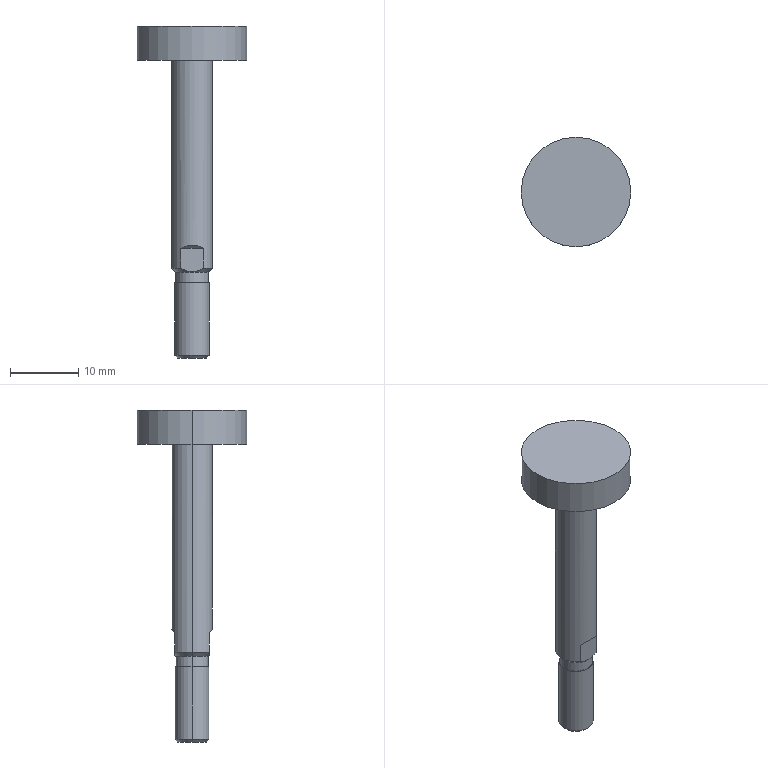Part | NX | features BREP 1 | 1 solid | 20 faces | box 16 x 16 x 48.5 mm | volume 2113 mm3 | cylinder 8 | plane 8 | cone 4 | commonest cylinder face diameters 4.8 x2 5 x2 6 x2 16 x2
STEP:
#1=CARTESIAN_POINT('',(2.1,0.,-43.5));
#2=VERTEX_POINT('',#1);
#3=CARTESIAN_POINT('',(-2.1,0.,-43.5));
#4=VERTEX_POINT('',#3);
#5=CARTESIAN_POINT('',(0.,0.,-43.5));
#6=DIRECTION('',(0.,0.,1.));
#7=DIRECTION('',(1.,0.,0.));
#8=AXIS2_PLACEMENT_3D('',#5,#6,#7);
#9=CIRCLE('',#8,2.1);
#10=EDGE_CURVE('',#2,#4,#9,.T.);
#11=ORIENTED_EDGE('',*,*,#10,.T.);
#12=CARTESIAN_POINT('',(-2.5,0.,-43.1));
#13=VERTEX_POINT('',#12);
#14=CARTESIAN_POINT('',(-2.5,0.,-43.1));
#15=DIRECTION('',(-0.7071,0.,0.7071));
#16=VECTOR('',#15,1000.);
#17=LINE('',#14,#16);
#18=EDGE_CURVE('',#13,#4,#17,.F.);
#19=ORIENTED_EDGE('',*,*,#18,.F.);
#20=CARTESIAN_POINT('',(2.5,0.,-43.1));
#21=VERTEX_POINT('',#20);
#22=CARTESIAN_POINT('',(0.,0.,-43.1));
#23=DIRECTION('',(0.,0.,1.));
#24=DIRECTION('',(1.,0.,0.));
#25=AXIS2_PLACEMENT_3D('',#22,#23,#24);
#26=CIRCLE('',#25,2.5);
#27=EDGE_CURVE('',#21,#13,#26,.T.);
#28=ORIENTED_EDGE('',*,*,#27,.F.);
#29=CARTESIAN_POINT('',(2.5,0.,-43.1));
#30=DIRECTION('',(0.7071,0.,0.7071));
#31=VECTOR('',#30,1000.);
#32=LINE('',#29,#31);
#33=EDGE_CURVE('',#21,#2,#32,.F.);
#34=ORIENTED_EDGE('',*,*,#33,.T.);
#35=EDGE_LOOP('',(#11,#19,#28,#34));
#36=FACE_BOUND('',#35,.T.);
#37=CARTESIAN_POINT('',(0.,0.,-43.1));
#38=DIRECTION('',(0.,0.,1.));
#39=DIRECTION('',(1.,0.,0.));
#40=AXIS2_PLACEMENT_3D('',#37,#38,#39);
#41=CONICAL_SURFACE('',#40,2.5,0.7854);
#42=ADVANCED_FACE('',(#36),#41,.T.);
#43=ORIENTED_EDGE('',*,*,#27,.T.);
#44=CARTESIAN_POINT('',(-2.5,0.,-32.5));
#45=VERTEX_POINT('',#44);
#46=CARTESIAN_POINT('',(-2.5,0.,0.));
#47=DIRECTION('',(0.,0.,1.));
#48=VECTOR('',#47,1000.);
#49=LINE('',#46,#48);
#50=EDGE_CURVE('',#45,#13,#49,.F.);
#51=ORIENTED_EDGE('',*,*,#50,.F.);
#52=CARTESIAN_POINT('',(2.5,0.,-32.5));
#53=VERTEX_POINT('',#52);
#54=CARTESIAN_POINT('',(0.,0.,-32.5));
#55=DIRECTION('',(0.,0.,1.));
#56=DIRECTION('',(1.,0.,0.));
#57=AXIS2_PLACEMENT_3D('',#54,#55,#56);
#58=CIRCLE('',#57,2.5);
#59=EDGE_CURVE('',#53,#45,#58,.T.);
#60=ORIENTED_EDGE('',*,*,#59,.F.);
#61=CARTESIAN_POINT('',(2.5,0.,0.));
#62=DIRECTION('',(0.,0.,1.));
#63=VECTOR('',#62,1000.);
#64=LINE('',#61,#63);
#65=EDGE_CURVE('',#53,#21,#64,.F.);
#66=ORIENTED_EDGE('',*,*,#65,.T.);
#67=EDGE_LOOP('',(#43,#51,#60,#66));
#68=FACE_BOUND('',#67,.T.);
#69=CARTESIAN_POINT('',(0.,0.,0.));
#70=DIRECTION('',(0.,0.,1.));
#71=DIRECTION('',(1.,0.,0.));
#72=AXIS2_PLACEMENT_3D('',#69,#70,#71);
#73=CYLINDRICAL_SURFACE('',#72,2.5);
#74=ADVANCED_FACE('',(#68),#73,.T.);
#75=CARTESIAN_POINT('',(2.4,0.,-32.5));
#76=VERTEX_POINT('',#75);
#77=CARTESIAN_POINT('',(-2.4,0.,-32.5));
#78=VERTEX_POINT('',#77);
#79=CARTESIAN_POINT('',(0.,0.,-32.5));
#80=DIRECTION('',(0.,0.,1.));
#81=DIRECTION('',(1.,0.,0.));
#82=AXIS2_PLACEMENT_3D('',#79,#80,#81);
#83=CIRCLE('',#82,2.4);
#84=EDGE_CURVE('',#76,#78,#83,.T.);
#85=ORIENTED_EDGE('',*,*,#84,.T.);
#86=CARTESIAN_POINT('',(-2.4,0.,-31.));
#87=VERTEX_POINT('',#86);
#88=CARTESIAN_POINT('',(-2.4,0.,0.));
#89=DIRECTION('',(0.,0.,1.));
#90=VECTOR('',#89,1000.);
#91=LINE('',#88,#90);
#92=EDGE_CURVE('',#87,#78,#91,.F.);
#93=ORIENTED_EDGE('',*,*,#92,.F.);
#94=CARTESIAN_POINT('',(2.4,0.,-31.));
#95=VERTEX_POINT('',#94);
#96=CARTESIAN_POINT('',(0.,0.,-31.));
#97=DIRECTION('',(0.,0.,1.));
#98=DIRECTION('',(1.,0.,0.));
#99=AXIS2_PLACEMENT_3D('',#96,#97,#98);
#100=CIRCLE('',#99,2.4);
#101=EDGE_CURVE('',#95,#87,#100,.T.);
#102=ORIENTED_EDGE('',*,*,#101,.F.);
#103=CARTESIAN_POINT('',(2.4,0.,0.));
#104=DIRECTION('',(0.,0.,1.));
#105=VECTOR('',#104,1000.);
#106=LINE('',#103,#105);
#107=EDGE_CURVE('',#95,#76,#106,.F.);
#108=ORIENTED_EDGE('',*,*,#107,.T.);
#109=EDGE_LOOP('',(#85,#93,#102,#108));
#110=FACE_BOUND('',#109,.T.);
#111=CARTESIAN_POINT('',(0.,0.,0.));
#112=DIRECTION('',(0.,0.,1.));
#113=DIRECTION('',(1.,0.,0.));
#114=AXIS2_PLACEMENT_3D('',#111,#112,#113);
#115=CYLINDRICAL_SURFACE('',#114,2.4);
#116=ADVANCED_FACE('',(#110),#115,.T.);
#117=ORIENTED_EDGE('',*,*,#101,.T.);
#118=CARTESIAN_POINT('',(-3.,0.,-30.4));
#119=VERTEX_POINT('',#118);
#120=CARTESIAN_POINT('',(-8.,0.,-25.4));
#121=DIRECTION('',(-0.7071,0.,0.7071));
#122=VECTOR('',#121,1000.);
#123=LINE('',#120,#122);
#124=EDGE_CURVE('',#119,#87,#123,.F.);
#125=ORIENTED_EDGE('',*,*,#124,.F.);
#126=CARTESIAN_POINT('',(-1.658,2.5,-30.4));
#127=VERTEX_POINT('',#126);
#128=CARTESIAN_POINT('',(0.,0.,-30.4));
#129=DIRECTION('',(0.,0.,1.));
#130=DIRECTION('',(1.,0.,0.));
#131=AXIS2_PLACEMENT_3D('',#128,#129,#130);
#132=CIRCLE('',#131,3.);
#133=EDGE_CURVE('',#127,#119,#132,.T.);
#134=ORIENTED_EDGE('',*,*,#133,.F.);
#135=CARTESIAN_POINT('',(1.658,2.5,-30.4));
#136=VERTEX_POINT('',#135);
#137=CARTESIAN_POINT('',(1.658,2.5,-30.4));
#138=CARTESIAN_POINT('',(1.376,2.5,-30.556));
#139=CARTESIAN_POINT('',(0.8861,2.5,-30.784));
#140=CARTESIAN_POINT('',(-0.001734,2.5,-30.958));
#141=CARTESIAN_POINT('',(-0.8871,2.5,-30.783));
#142=CARTESIAN_POINT('',(-1.376,2.5,-30.556));
#143=CARTESIAN_POINT('',(-1.658,2.5,-30.4));
#144=B_SPLINE_CURVE_WITH_KNOTS('',3,(#137,#138,#139,#140,#141,#142,#143),.UNSPECIFIED.,.F.,.F.,(4,1,1,1,4),(0.,0.25,0.5,0.75,1.),.UNSPECIFIED.);
#145=EDGE_CURVE('',#136,#127,#144,.T.);
#146=ORIENTED_EDGE('',*,*,#145,.F.);
#147=CARTESIAN_POINT('',(3.,0.,-30.4));
#148=VERTEX_POINT('',#147);
#149=CARTESIAN_POINT('',(0.,0.,-30.4));
#150=DIRECTION('',(0.,0.,1.));
#151=DIRECTION('',(1.,0.,0.));
#152=AXIS2_PLACEMENT_3D('',#149,#150,#151);
#153=CIRCLE('',#152,3.);
#154=EDGE_CURVE('',#148,#136,#153,.T.);
#155=ORIENTED_EDGE('',*,*,#154,.F.);
#156=CARTESIAN_POINT('',(8.,0.,-25.4));
#157=DIRECTION('',(0.7071,0.,0.7071));
#158=VECTOR('',#157,1000.);
#159=LINE('',#156,#158);
#160=EDGE_CURVE('',#148,#95,#159,.F.);
#161=ORIENTED_EDGE('',*,*,#160,.T.);
#162=EDGE_LOOP('',(#117,#125,#134,#146,#155,#161));
#163=FACE_BOUND('',#162,.T.);
#164=CARTESIAN_POINT('',(0.,0.,-25.4));
#165=DIRECTION('',(0.,0.,1.));
#166=DIRECTION('',(1.,0.,0.));
#167=AXIS2_PLACEMENT_3D('',#164,#165,#166);
#168=CONICAL_SURFACE('',#167,8.,0.7854);
#169=ADVANCED_FACE('',(#163),#168,.T.);
#170=CARTESIAN_POINT('',(8.,0.,5.));
#171=VERTEX_POINT('',#170);
#172=CARTESIAN_POINT('',(-8.,0.,5.));
#173=VERTEX_POINT('',#172);
#174=CARTESIAN_POINT('',(0.,0.,5.));
#175=DIRECTION('',(0.,0.,1.));
#176=DIRECTION('',(1.,0.,0.));
#177=AXIS2_PLACEMENT_3D('',#174,#175,#176);
#178=CIRCLE('',#177,8.);
#179=EDGE_CURVE('',#171,#173,#178,.T.);
#180=ORIENTED_EDGE('',*,*,#179,.F.);
#181=CARTESIAN_POINT('',(8.,0.,0.));
#182=VERTEX_POINT('',#181);
#183=CARTESIAN_POINT('',(8.,0.,5.));
#184=DIRECTION('',(0.,0.,-1.));
#185=VECTOR('',#184,1000.);
#186=LINE('',#183,#185);
#187=EDGE_CURVE('',#171,#182,#186,.T.);
#188=ORIENTED_EDGE('',*,*,#187,.T.);
#189=CARTESIAN_POINT('',(-8.,0.,0.));
#190=VERTEX_POINT('',#189);
#191=CARTESIAN_POINT('',(0.,0.,0.));
#192=DIRECTION('',(0.,0.,1.));
#193=DIRECTION('',(1.,0.,0.));
#194=AXIS2_PLACEMENT_3D('',#191,#192,#193);
#195=CIRCLE('',#194,8.);
#196=EDGE_CURVE('',#182,#190,#195,.T.);
#197=ORIENTED_EDGE('',*,*,#196,.T.);
#198=CARTESIAN_POINT('',(-8.,0.,5.));
#199=DIRECTION('',(0.,0.,-1.));
#200=VECTOR('',#199,1000.);
#201=LINE('',#198,#200);
#202=EDGE_CURVE('',#173,#190,#201,.T.);
#203=ORIENTED_EDGE('',*,*,#202,.F.);
#204=EDGE_LOOP('',(#180,#188,#197,#203));
#205=FACE_BOUND('',#204,.T.);
#206=CARTESIAN_POINT('',(0.,0.,5.));
#207=DIRECTION('',(0.,0.,-1.));
#208=DIRECTION('',(-1.,0.,0.));
#209=AXIS2_PLACEMENT_3D('',#206,#207,#208);
#210=CYLINDRICAL_SURFACE('',#209,8.);
#211=ADVANCED_FACE('',(#205),#210,.T.);
#212=ORIENTED_EDGE('',*,*,#133,.T.);
#213=CARTESIAN_POINT('',(-3.,0.,0.));
#214=VERTEX_POINT('',#213);
#215=CARTESIAN_POINT('',(-3.,0.,-51.985));
#216=DIRECTION('',(0.,0.,1.));
#217=VECTOR('',#216,1000.);
#218=LINE('',#215,#217);
#219=EDGE_CURVE('',#214,#119,#218,.F.);
#220=ORIENTED_EDGE('',*,*,#219,.F.);
#221=CARTESIAN_POINT('',(3.,0.,0.));
#222=VERTEX_POINT('',#221);
#223=CARTESIAN_POINT('',(0.,0.,0.));
#224=DIRECTION('',(0.,0.,1.));
#225=DIRECTION('',(1.,0.,0.));
#226=AXIS2_PLACEMENT_3D('',#223,#224,#225);
#227=CIRCLE('',#226,3.);
#228=EDGE_CURVE('',#222,#214,#227,.T.);
#229=ORIENTED_EDGE('',*,*,#228,.F.);
#230=CARTESIAN_POINT('',(3.,0.,-51.985));
#231=DIRECTION('',(0.,0.,1.));
#232=VECTOR('',#231,1000.);
#233=LINE('',#230,#232);
#234=EDGE_CURVE('',#222,#148,#233,.F.);
#235=ORIENTED_EDGE('',*,*,#234,.T.);
#236=ORIENTED_EDGE('',*,*,#154,.T.);
#237=CARTESIAN_POINT('',(1.658,2.5,-27.5));
#238=VERTEX_POINT('',#237);
#239=CARTESIAN_POINT('',(1.658,2.5,-51.985));
#240=DIRECTION('',(0.,0.,-1.));
#241=VECTOR('',#240,1000.);
#242=LINE('',#239,#241);
#243=EDGE_CURVE('',#238,#136,#242,.T.);
#244=ORIENTED_EDGE('',*,*,#243,.F.);
#245=CARTESIAN_POINT('',(-1.658,2.5,-27.5));
#246=VERTEX_POINT('',#245);
#247=CARTESIAN_POINT('',(-1.658,2.5,-27.5));
#248=CARTESIAN_POINT('',(-0.6219,3.188,-26.812));
#249=CARTESIAN_POINT('',(0.6219,3.188,-26.812));
#250=CARTESIAN_POINT('',(1.658,2.5,-27.5));
#251=(BOUNDED_CURVE()B_SPLINE_CURVE(3,(#247,#248,#249,#250),.UNSPECIFIED.,.F.,.F.)B_SPLINE_CURVE_WITH_KNOTS((4,4),(5.697,6.869),.UNSPECIFIED.)CURVE()GEOMETRIC_REPRESENTATION_ITEM()RATIONAL_B_SPLINE_CURVE((1.,0.8889,0.8889,1.))REPRESENTATION_ITEM(''));
#252=EDGE_CURVE('',#246,#238,#251,.T.);
#253=ORIENTED_EDGE('',*,*,#252,.F.);
#254=CARTESIAN_POINT('',(-1.658,2.5,-51.985));
#255=DIRECTION('',(0.,0.,1.));
#256=VECTOR('',#255,1000.);
#257=LINE('',#254,#256);
#258=EDGE_CURVE('',#127,#246,#257,.T.);
#259=ORIENTED_EDGE('',*,*,#258,.F.);
#260=EDGE_LOOP('',(#212,#220,#229,#235,#236,#244,#253,#259));
#261=FACE_BOUND('',#260,.T.);
#262=CARTESIAN_POINT('',(0.,0.,-51.985));
#263=DIRECTION('',(0.,0.,1.));
#264=DIRECTION('',(1.,0.,0.));
#265=AXIS2_PLACEMENT_3D('',#262,#263,#264);
#266=CYLINDRICAL_SURFACE('',#265,3.);
#267=ADVANCED_FACE('',(#261),#266,.T.);
#268=ORIENTED_EDGE('',*,*,#219,.T.);
#269=CARTESIAN_POINT('',(-1.658,-2.5,-30.4));
#270=VERTEX_POINT('',#269);
#271=CARTESIAN_POINT('',(0.,0.,-30.4));
#272=DIRECTION('',(0.,0.,1.));
#273=DIRECTION('',(1.,0.,0.));
#274=AXIS2_PLACEMENT_3D('',#271,#272,#273);
#275=CIRCLE('',#274,3.);
#276=EDGE_CURVE('',#119,#270,#275,.T.);
#277=ORIENTED_EDGE('',*,*,#276,.T.);
#278=CARTESIAN_POINT('',(-1.658,-2.5,-27.5));
#279=VERTEX_POINT('',#278);
#280=CARTESIAN_POINT('',(-1.658,-2.5,-51.985));
#281=DIRECTION('',(0.,0.,-1.));
#282=VECTOR('',#281,1000.);
#283=LINE('',#280,#282);
#284=EDGE_CURVE('',#279,#270,#283,.T.);
#285=ORIENTED_EDGE('',*,*,#284,.F.);
#286=CARTESIAN_POINT('',(1.658,-2.5,-27.5));
#287=VERTEX_POINT('',#286);
#288=CARTESIAN_POINT('',(1.658,-2.5,-27.5));
#289=CARTESIAN_POINT('',(0.6219,-3.188,-26.812));
#290=CARTESIAN_POINT('',(-0.6219,-3.188,-26.812));
#291=CARTESIAN_POINT('',(-1.658,-2.5,-27.5));
#292=(BOUNDED_CURVE()B_SPLINE_CURVE(3,(#288,#289,#290,#291),.UNSPECIFIED.,.F.,.F.)B_SPLINE_CURVE_WITH_KNOTS((4,4),(5.697,6.869),.UNSPECIFIED.)CURVE()GEOMETRIC_REPRESENTATION_ITEM()RATIONAL_B_SPLINE_CURVE((1.,0.8889,0.8889,1.))REPRESENTATION_ITEM(''));
#293=EDGE_CURVE('',#287,#279,#292,.T.);
#294=ORIENTED_EDGE('',*,*,#293,.F.);
#295=CARTESIAN_POINT('',(1.658,-2.5,-30.4));
#296=VERTEX_POINT('',#295);
#297=CARTESIAN_POINT('',(1.658,-2.5,-51.985));
#298=DIRECTION('',(0.,0.,1.));
#299=VECTOR('',#298,1000.);
#300=LINE('',#297,#299);
#301=EDGE_CURVE('',#296,#287,#300,.T.);
#302=ORIENTED_EDGE('',*,*,#301,.F.);
#303=CARTESIAN_POINT('',(0.,0.,-30.4));
#304=DIRECTION('',(0.,0.,1.));
#305=DIRECTION('',(1.,0.,0.));
#306=AXIS2_PLACEMENT_3D('',#303,#304,#305);
#307=CIRCLE('',#306,3.);
#308=EDGE_CURVE('',#296,#148,#307,.T.);
#309=ORIENTED_EDGE('',*,*,#308,.T.);
#310=ORIENTED_EDGE('',*,*,#234,.F.);
#311=CARTESIAN_POINT('',(0.,0.,0.));
#312=DIRECTION('',(0.,0.,1.));
#313=DIRECTION('',(1.,0.,0.));
#314=AXIS2_PLACEMENT_3D('',#311,#312,#313);
#315=CIRCLE('',#314,3.);
#316=EDGE_CURVE('',#214,#222,#315,.T.);
#317=ORIENTED_EDGE('',*,*,#316,.F.);
#318=EDGE_LOOP('',(#268,#277,#285,#294,#302,#309,#310,#317));
#319=FACE_BOUND('',#318,.T.);
#320=CARTESIAN_POINT('',(0.,0.,-51.985));
#321=DIRECTION('',(0.,0.,1.));
#322=DIRECTION('',(1.,0.,0.));
#323=AXIS2_PLACEMENT_3D('',#320,#321,#322);
#324=CYLINDRICAL_SURFACE('',#323,3.);
#325=ADVANCED_FACE('',(#319),#324,.T.);
#326=ORIENTED_EDGE('',*,*,#187,.F.);
#327=CARTESIAN_POINT('',(0.,0.,5.));
#328=DIRECTION('',(0.,0.,1.));
#329=DIRECTION('',(1.,0.,0.));
#330=AXIS2_PLACEMENT_3D('',#327,#328,#329);
#331=CIRCLE('',#330,8.);
#332=EDGE_CURVE('',#173,#171,#331,.T.);
#333=ORIENTED_EDGE('',*,*,#332,.F.);
#334=ORIENTED_EDGE('',*,*,#202,.T.);
#335=CARTESIAN_POINT('',(0.,0.,0.));
#336=DIRECTION('',(0.,0.,1.));
#337=DIRECTION('',(1.,0.,0.));
#338=AXIS2_PLACEMENT_3D('',#335,#336,#337);
#339=CIRCLE('',#338,8.);
#340=EDGE_CURVE('',#190,#182,#339,.T.);
#341=ORIENTED_EDGE('',*,*,#340,.T.);
#342=EDGE_LOOP('',(#326,#333,#334,#341));
#343=FACE_BOUND('',#342,.T.);
#344=CARTESIAN_POINT('',(0.,0.,5.));
#345=DIRECTION('',(0.,0.,-1.));
#346=DIRECTION('',(-1.,0.,0.));
#347=AXIS2_PLACEMENT_3D('',#344,#345,#346);
#348=CYLINDRICAL_SURFACE('',#347,8.);
#349=ADVANCED_FACE('',(#343),#348,.T.);
#350=ORIENTED_EDGE('',*,*,#332,.T.);
#351=ORIENTED_EDGE('',*,*,#179,.T.);
#352=EDGE_LOOP('',(#350,#351));
#353=FACE_BOUND('',#352,.T.);
#354=CARTESIAN_POINT('',(0.,0.,5.));
#355=DIRECTION('',(0.,0.,1.));
#356=DIRECTION('',(1.,0.,0.));
#357=AXIS2_PLACEMENT_3D('',#354,#355,#356);
#358=PLANE('',#357);
#359=ADVANCED_FACE('',(#353),#358,.T.);
#360=ORIENTED_EDGE('',*,*,#340,.F.);
#361=ORIENTED_EDGE('',*,*,#196,.F.);
#362=EDGE_LOOP('',(#360,#361));
#363=FACE_BOUND('',#362,.T.);
#364=ORIENTED_EDGE('',*,*,#228,.T.);
#365=ORIENTED_EDGE('',*,*,#316,.T.);
#366=EDGE_LOOP('',(#364,#365));
#367=FACE_BOUND('',#366,.T.);
#368=CARTESIAN_POINT('',(0.,0.,0.));
#369=DIRECTION('',(0.,0.,1.));
#370=DIRECTION('',(1.,0.,0.));
#371=AXIS2_PLACEMENT_3D('',#368,#369,#370);
#372=PLANE('',#371);
#373=ADVANCED_FACE('',(#363,#367),#372,.F.);
#374=ORIENTED_EDGE('',*,*,#124,.T.);
#375=CARTESIAN_POINT('',(0.,0.,-31.));
#376=DIRECTION('',(0.,0.,1.));
#377=DIRECTION('',(1.,0.,0.));
#378=AXIS2_PLACEMENT_3D('',#375,#376,#377);
#379=CIRCLE('',#378,2.4);
#380=EDGE_CURVE('',#87,#95,#379,.T.);
#381=ORIENTED_EDGE('',*,*,#380,.T.);
#382=ORIENTED_EDGE('',*,*,#160,.F.);
#383=ORIENTED_EDGE('',*,*,#308,.F.);
#384=CARTESIAN_POINT('',(-1.658,-2.5,-30.4));
#385=CARTESIAN_POINT('',(-1.376,-2.5,-30.556));
#386=CARTESIAN_POINT('',(-0.8867,-2.5,-30.783));
#387=CARTESIAN_POINT('',(-0.001927,-2.5,-30.958));
#388=CARTESIAN_POINT('',(0.8864,-2.5,-30.784));
#389=CARTESIAN_POINT('',(1.375,-2.5,-30.557));
#390=CARTESIAN_POINT('',(1.658,-2.5,-30.4));
#391=B_SPLINE_CURVE_WITH_KNOTS('',3,(#384,#385,#386,#387,#388,#389,#390),.UNSPECIFIED.,.F.,.F.,(4,1,1,1,4),(0.,0.25,0.5,0.75,1.),.UNSPECIFIED.);
#392=EDGE_CURVE('',#270,#296,#391,.T.);
#393=ORIENTED_EDGE('',*,*,#392,.F.);
#394=ORIENTED_EDGE('',*,*,#276,.F.);
#395=EDGE_LOOP('',(#374,#381,#382,#383,#393,#394));
#396=FACE_BOUND('',#395,.T.);
#397=CARTESIAN_POINT('',(0.,0.,-25.4));
#398=DIRECTION('',(0.,0.,1.));
#399=DIRECTION('',(1.,0.,0.));
#400=AXIS2_PLACEMENT_3D('',#397,#398,#399);
#401=CONICAL_SURFACE('',#400,8.,0.7854);
#402=ADVANCED_FACE('',(#396),#401,.T.);
#403=ORIENTED_EDGE('',*,*,#92,.T.);
#404=CARTESIAN_POINT('',(0.,0.,-32.5));
#405=DIRECTION('',(0.,0.,1.));
#406=DIRECTION('',(1.,0.,0.));
#407=AXIS2_PLACEMENT_3D('',#404,#405,#406);
#408=CIRCLE('',#407,2.4);
#409=EDGE_CURVE('',#78,#76,#408,.T.);
#410=ORIENTED_EDGE('',*,*,#409,.T.);
#411=ORIENTED_EDGE('',*,*,#107,.F.);
#412=ORIENTED_EDGE('',*,*,#380,.F.);
#413=EDGE_LOOP('',(#403,#410,#411,#412));
#414=FACE_BOUND('',#413,.T.);
#415=CARTESIAN_POINT('',(0.,0.,0.));
#416=DIRECTION('',(0.,0.,1.));
#417=DIRECTION('',(1.,0.,0.));
#418=AXIS2_PLACEMENT_3D('',#415,#416,#417);
#419=CYLINDRICAL_SURFACE('',#418,2.4);
#420=ADVANCED_FACE('',(#414),#419,.T.);
#421=ORIENTED_EDGE('',*,*,#59,.T.);
#422=CARTESIAN_POINT('',(0.,0.,-32.5));
#423=DIRECTION('',(0.,0.,1.));
#424=DIRECTION('',(1.,0.,0.));
#425=AXIS2_PLACEMENT_3D('',#422,#423,#424);
#426=CIRCLE('',#425,2.5);
#427=EDGE_CURVE('',#45,#53,#426,.T.);
#428=ORIENTED_EDGE('',*,*,#427,.T.);
#429=EDGE_LOOP('',(#421,#428));
#430=FACE_BOUND('',#429,.T.);
#431=ORIENTED_EDGE('',*,*,#84,.F.);
#432=ORIENTED_EDGE('',*,*,#409,.F.);
#433=EDGE_LOOP('',(#431,#432));
#434=FACE_BOUND('',#433,.T.);
#435=CARTESIAN_POINT('',(0.,2.5,-32.5));
#436=DIRECTION('',(0.,0.,1.));
#437=DIRECTION('',(1.,0.,0.));
#438=AXIS2_PLACEMENT_3D('',#435,#436,#437);
#439=PLANE('',#438);
#440=ADVANCED_FACE('',(#430,#434),#439,.T.);
#441=ORIENTED_EDGE('',*,*,#50,.T.);
#442=CARTESIAN_POINT('',(0.,0.,-43.1));
#443=DIRECTION('',(0.,0.,1.));
#444=DIRECTION('',(1.,0.,0.));
#445=AXIS2_PLACEMENT_3D('',#442,#443,#444);
#446=CIRCLE('',#445,2.5);
#447=EDGE_CURVE('',#13,#21,#446,.T.);
#448=ORIENTED_EDGE('',*,*,#447,.T.);
#449=ORIENTED_EDGE('',*,*,#65,.F.);
#450=ORIENTED_EDGE('',*,*,#427,.F.);
#451=EDGE_LOOP('',(#441,#448,#449,#450));
#452=FACE_BOUND('',#451,.T.);
#453=CARTESIAN_POINT('',(0.,0.,0.));
#454=DIRECTION('',(0.,0.,1.));
#455=DIRECTION('',(1.,0.,0.));
#456=AXIS2_PLACEMENT_3D('',#453,#454,#455);
#457=CYLINDRICAL_SURFACE('',#456,2.5);
#458=ADVANCED_FACE('',(#452),#457,.T.);
#459=ORIENTED_EDGE('',*,*,#18,.T.);
#460=CARTESIAN_POINT('',(0.,0.,-43.5));
#461=DIRECTION('',(0.,0.,1.));
#462=DIRECTION('',(1.,0.,0.));
#463=AXIS2_PLACEMENT_3D('',#460,#461,#462);
#464=CIRCLE('',#463,2.1);
#465=EDGE_CURVE('',#4,#2,#464,.T.);
#466=ORIENTED_EDGE('',*,*,#465,.T.);
#467=ORIENTED_EDGE('',*,*,#33,.F.);
#468=ORIENTED_EDGE('',*,*,#447,.F.);
#469=EDGE_LOOP('',(#459,#466,#467,#468));
#470=FACE_BOUND('',#469,.T.);
#471=CARTESIAN_POINT('',(0.,0.,-43.1));
#472=DIRECTION('',(0.,0.,1.));
#473=DIRECTION('',(1.,0.,0.));
#474=AXIS2_PLACEMENT_3D('',#471,#472,#473);
#475=CONICAL_SURFACE('',#474,2.5,0.7854);
#476=ADVANCED_FACE('',(#470),#475,.T.);
#477=ORIENTED_EDGE('',*,*,#10,.F.);
#478=ORIENTED_EDGE('',*,*,#465,.F.);
#479=EDGE_LOOP('',(#477,#478));
#480=FACE_BOUND('',#479,.T.);
#481=CARTESIAN_POINT('',(0.,0.,-43.5));
#482=DIRECTION('',(0.,0.,1.));
#483=DIRECTION('',(1.,0.,0.));
#484=AXIS2_PLACEMENT_3D('',#481,#482,#483);
#485=PLANE('',#484);
#486=ADVANCED_FACE('',(#480),#485,.F.);
#487=ORIENTED_EDGE('',*,*,#243,.T.);
#488=ORIENTED_EDGE('',*,*,#145,.T.);
#489=ORIENTED_EDGE('',*,*,#258,.T.);
#490=CARTESIAN_POINT('',(-8.,2.5,-27.5));
#491=DIRECTION('',(1.,0.,0.));
#492=VECTOR('',#491,1000.);
#493=LINE('',#490,#492);
#494=EDGE_CURVE('',#246,#238,#493,.T.);
#495=ORIENTED_EDGE('',*,*,#494,.T.);
#496=EDGE_LOOP('',(#487,#488,#489,#495));
#497=FACE_BOUND('',#496,.T.);
#498=CARTESIAN_POINT('',(-8.,2.5,-43.5));
#499=DIRECTION('',(0.,-1.,0.));
#500=DIRECTION('',(0.,0.,-1.));
#501=AXIS2_PLACEMENT_3D('',#498,#499,#500);
#502=PLANE('',#501);
#503=ADVANCED_FACE('',(#497),#502,.F.);
#504=ORIENTED_EDGE('',*,*,#252,.T.);
#505=ORIENTED_EDGE('',*,*,#494,.F.);
#506=EDGE_LOOP('',(#504,#505));
#507=FACE_BOUND('',#506,.T.);
#508=CARTESIAN_POINT('',(-8.,2.5,-27.5));
#509=DIRECTION('',(0.,-0.7071,0.7071));
#510=DIRECTION('',(-1.,0.,0.));
#511=AXIS2_PLACEMENT_3D('',#508,#509,#510);
#512=PLANE('',#511);
#513=ADVANCED_FACE('',(#507),#512,.F.);
#514=ORIENTED_EDGE('',*,*,#293,.T.);
#515=CARTESIAN_POINT('',(-8.,-2.5,-27.5));
#516=DIRECTION('',(1.,0.,0.));
#517=VECTOR('',#516,1000.);
#518=LINE('',#515,#517);
#519=EDGE_CURVE('',#279,#287,#518,.T.);
#520=ORIENTED_EDGE('',*,*,#519,.T.);
#521=EDGE_LOOP('',(#514,#520));
#522=FACE_BOUND('',#521,.T.);
#523=CARTESIAN_POINT('',(-8.,-2.5,-27.5));
#524=DIRECTION('',(0.,0.7071,0.7071));
#525=DIRECTION('',(1.,0.,0.));
#526=AXIS2_PLACEMENT_3D('',#523,#524,#525);
#527=PLANE('',#526);
#528=ADVANCED_FACE('',(#522),#527,.F.);
#529=ORIENTED_EDGE('',*,*,#284,.T.);
#530=ORIENTED_EDGE('',*,*,#392,.T.);
#531=ORIENTED_EDGE('',*,*,#301,.T.);
#532=ORIENTED_EDGE('',*,*,#519,.F.);
#533=EDGE_LOOP('',(#529,#530,#531,#532));
#534=FACE_BOUND('',#533,.T.);
#535=CARTESIAN_POINT('',(-8.,-2.5,-43.5));
#536=DIRECTION('',(0.,1.,0.));
#537=DIRECTION('',(0.,0.,-1.));
#538=AXIS2_PLACEMENT_3D('',#535,#536,#537);
#539=PLANE('',#538);
#540=ADVANCED_FACE('',(#534),#539,.F.);
#541=CLOSED_SHELL('',(#42,#74,#116,#169,#211,#267,#325,#349,#359,#373,#402,#420,#440,#458,#476,#486,#503,#513,#528,#540));
#542=MANIFOLD_SOLID_BREP('',#541);
#543=(LENGTH_UNIT()NAMED_UNIT(*)SI_UNIT(.MILLI.,.METRE.));
#544=UNCERTAINTY_MEASURE_WITH_UNIT(LENGTH_MEASURE(0.0508),#543,'','');
#545=(NAMED_UNIT(*)PLANE_ANGLE_UNIT()SI_UNIT($,.RADIAN.));
#546=(NAMED_UNIT(*)SI_UNIT($,.STERADIAN.)SOLID_ANGLE_UNIT());
#547=(GEOMETRIC_REPRESENTATION_CONTEXT(3)GLOBAL_UNCERTAINTY_ASSIGNED_CONTEXT((#544))GLOBAL_UNIT_ASSIGNED_CONTEXT((#543,#545,#546))REPRESENTATION_CONTEXT('',''));
#548=ADVANCED_BREP_SHAPE_REPRESENTATION('',(#542),#547);